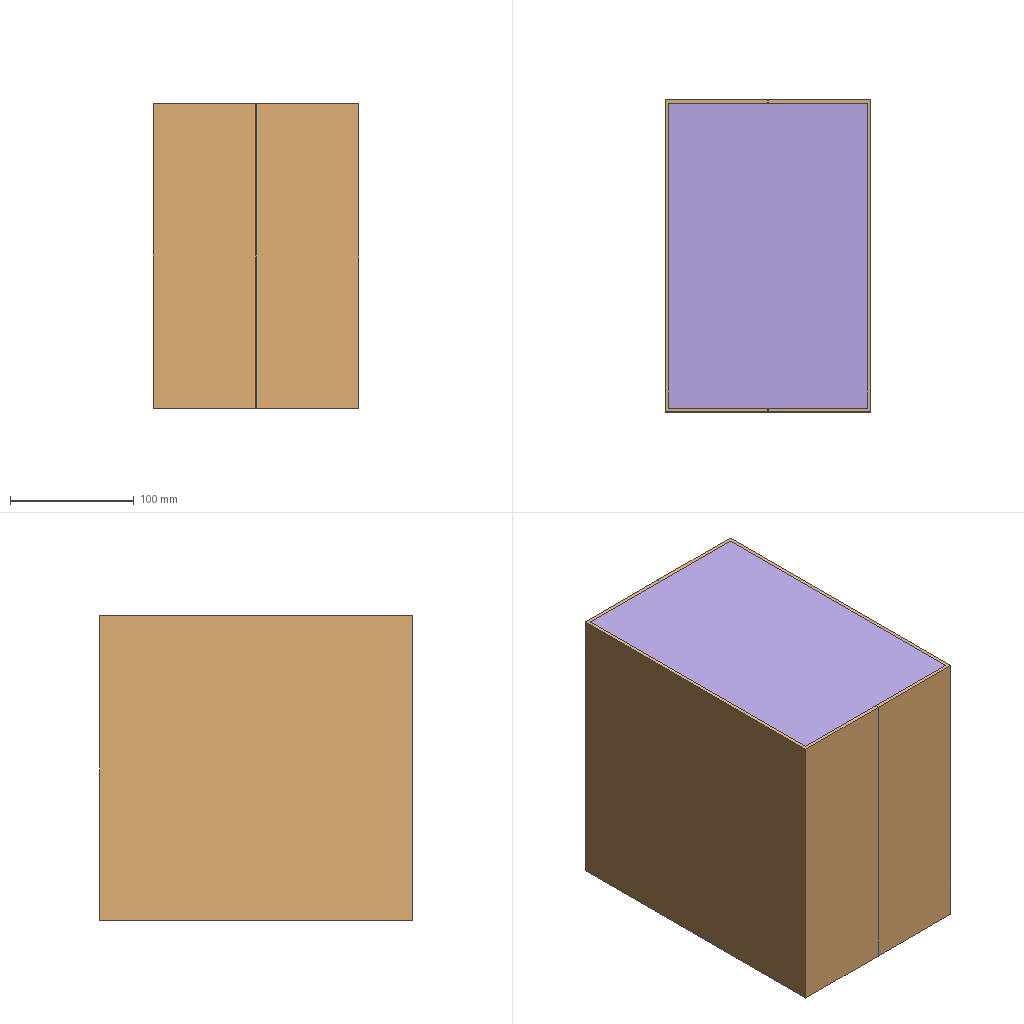Assembly | SolidWorks | 9 different items | 41 placed | box 166 x 252 x 246 mm
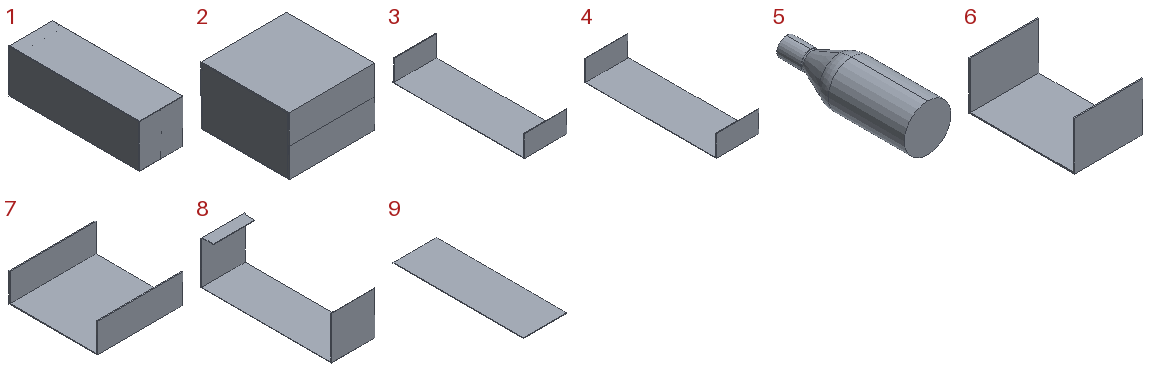Parts list (item | name | quantity | parent item | size | volume | features):
1 | (subassembly) | x6 | - | 80 x 240 x 80 mm | 101310 mm3 | -
2 | (subassembly) | x1 | - | 246 x 252 x 166 mm | 1055472 mm3 | -
3 | - | x6 | in 1 | 78 x 238 x 39 mm | 24455 mm3 | features ICE 2, Extrusion 1
4 | - | x6 | in 1 | 78 x 238 x 39 mm | 24455 mm3 | features ICE 2, Extrusion 1
5 | - | x6 | - | 78 x 236 x 78 mm | 361829 mm3 | features ICE 2, Revolution 1
6 | - | x2 | in 2 | 160 x 246 x 113 mm | 223680 mm3 | features Extrusion 1, ICE 1
7 | - | x2 | in 2 | 246 x 252 x 83 mm | 304056 mm3 | features Extrusion 1, ICE 1
8 | - | x6 | in 1 | 80 x 240 x 79 mm | 33200 mm3 | features ICE 3, Extrusion 1
9 | - | x6 | in 1 | 80 x 240 x 1 mm | 19200 mm3 | features Extrusion 1
Mates (type | each side: item.copy, entity, surface, feature):
In the top assembly
Coincident | 4.1 face plane Boss-Extrude2 | 5.1 face plane Revolve1
Symmetric | 9.1 face plane Boss-Extrude1 | 8.1 face plane Boss-Extrude1 | 5.1 plane
Symmetric | 3.1 face plane Boss-Extrude1 | 4.1 face plane Boss-Extrude1 | 5.1 plane
Coincident | 8.2 face plane Boss-Extrude1 | 6.1 face plane Boss-Extrude2
Width | 6.2 face plane Boss-Extrude1 | 6.1 face plane Boss-Extrude1 | 8.3 face plane Boss-Extrude1 | 9.2 face plane Boss-Extrude1
Width | 7.1 face plane Boss-Extrude1 | 7.2 face plane Boss-Extrude1 | 4.2 face plane Boss-Extrude1 | 3.2 face plane Boss-Extrude1
In subassembly 1
Coincident | 8.4 plane | 1.1 plane | 3 times
Coincident | 8.4 face plane Boss-Extrude2 | 3.3 face plane Boss-Extrude1
Coincident | 8.4 face plane Boss-Extrude1 | 3.3 face plane Boss-Extrude1 | 2 times
Coincident | 8.4 face plane Boss-Extrude2 | 9.3 face plane Boss-Extrude1
Coincident | 8.4 face plane Boss-Extrude1 | 9.3 face plane Boss-Extrude1 | 2 times
Coincident | 8.4 face plane Boss-Extrude1 | 4.3 face plane Boss-Extrude1 | 2 times
Coincident | 8.4 face plane Boss-Extrude2 | 4.3 face plane Boss-Extrude1
In subassembly 2
Coincident | 7.3 face plane Boss-Extrude1 | 7.4 face plane Boss-Extrude1 | 2 times
Coincident | 7.3 face plane Boss-Extrude2 | 7.4 face plane Boss-Extrude2
Coincident | 7.4 face plane Boss-Extrude1 | 6.3 face plane Boss-Extrude1
Coincident | 7.4 face plane Boss-Extrude2 | 6.3 face plane Boss-Extrude1
Coincident | 7.3 face plane Boss-Extrude1 | 6.3 face plane Boss-Extrude1
Coincident | 7.4 face plane Boss-Extrude2 | 6.4 face plane Boss-Extrude1
Coincident | 7.3 face plane Boss-Extrude1 | 6.4 face plane Boss-Extrude1
Coincident | 7.4 face plane Boss-Extrude1 | 6.4 face plane Boss-Extrude1